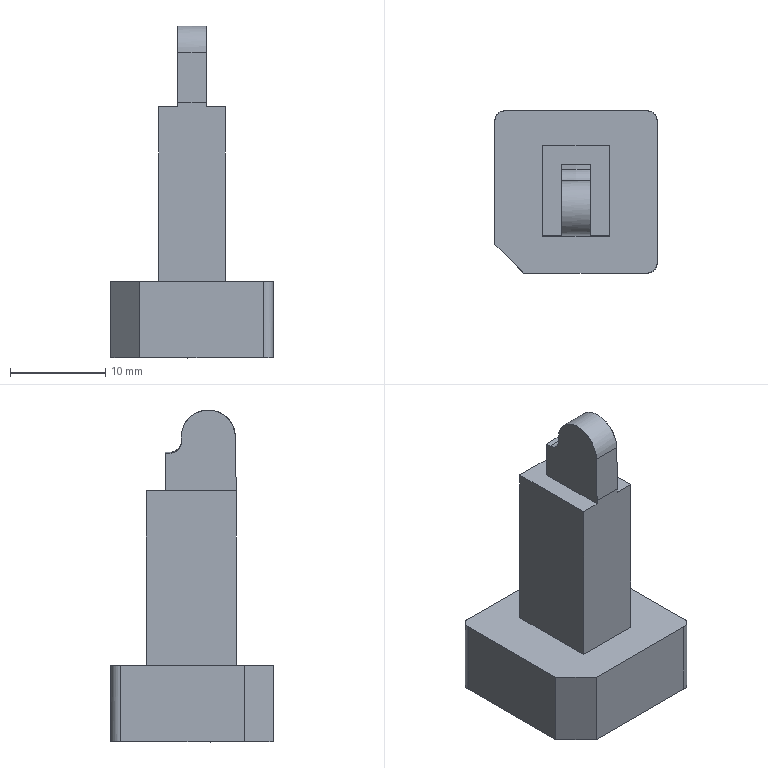NC program | PowerMill | posted with a generic post | part box 17 x 17 x 34.811 mm
Lines 1 to 1077 of 55221:
%
O0001
N104 ( POWERMILL CB  : 2026004.0)
N105 ( POST VER      : 2026.0.0.5161)
N106 ( OPTION FILE   : FANUC)
N107 ( OUTPUT WORKPLANE : WORLD)
N108 (  )
N109 ( TOOL LIST )
N110 (---------------------------------------)
N111 ( NO. | ID        | DIA.| TIP RAD|LENGTH)
N112 (---------------------------------------)
N113 (    1|D10C_1_1_1 |10.0 |  0.0   |90.28 )
N114 (    3|D10_1_1_1  |10.0 |  0.0   |89.96 )
N115 (    4|R1_1_1     | 2.0 |  1.0   |59.84 )
N116 (   14|D4_1_1     | 4.0 |  0.0   |63.76 )
N117 (   13|TEXT_D4_1_1| 4.0 |  0.3   |82.08 )
N118 (---------------------------------------)
N119 (  )
N120 ( NUMBER OF TOOLPATHS: 10.0 )
N121 ( ESTIMATED PROGRAM DURATION: 0 HOURS 6 MIN 45 SEC)
N122 (  )
N123 G00 G21 G80 G40 G17
N124 G90
N125 G54
N126 G53 Z0.0
N127 (---------------)
N128 ( START TOOLPATH : 精公开粗01-扫面平行-D10C )
N129 (---------------)
N130 ( TOOL NO.    :1 )
N131 ( TOOL TYPE   : ENDMILL)
N132 ( TOOL ID     : D10C_1_1_1)
N133 ( TOOL DIA    : 10.0 LENGTH 90.28)
N134 T1
N135 M6
N136 S8000 M03
N137 G00 G90 X0.0 Y0.0
N138 G43 Z10.2 H1
N139
N140 G05 P10000 R4
N141 X11.28 Y11.28
N142 Z1.128
N143 G01 Z-0.072 F6000.0
N144 X-11.28 F10000.0
N145 Y5.64
N146 X11.28
N147 Y0.0
N148 X-11.28
N149 Y-5.64
N150 X11.28
N151 Y-11.28
N152 X-11.28
N153 X-16.28
N154 G00 Z10.2
N155 G05 P0
N156 (---------------)
N157 ( END TOOLPATH : 精公开粗01-扫面平行-D10C )
N158 (---------------)
N159 ( START TOOLPATH : 精公开粗01-外形偏置-D10C )
N160 (---------------)
N161 G00 X0.0 Y0.0915 Z9.878
N162 G05 P10000 R4
N163 X4.7475 Y-17.685
N164 Z0.6945
N165 G01 Z-0.5055 F6000.0
N166 Y-17.1575 F10000.0
N167 G03 X0.0 Y-12.41 I-4.7475 J0.0
N168 G01 X-10.286
N169 G02 X-11.286 Y-11.41 I0.0 J1.0
N170 G01 Y11.593
N171 G02 X-10.286 Y12.593 I1.0 J0.0
N172 G01 X10.286
N173 G02 X11.286 Y11.593 I0.0 J-1.0
N174 G01 Y-11.41
N175 G02 X10.286 Y-12.41 I-1.0 J0.0
N176 G01 X0.0
N177 Y-8.3254
N178 X-1.9336
N179 X-2.707 Y-8.2036
N180 X-3.4804 Y-7.9573
N181 X-4.1209 Y-7.6428
N182 X-5.0273 Y-6.986
N183 X-5.1508 Y-6.8693
N184 X-5.8007 Y-6.1132
N185 X-6.2618 Y-5.3225
N186 X-6.5583 Y-4.5491
N187 X-6.7288 Y-3.7756
N188 X-6.7867 Y-3.0022
N189 Y-0.6819
N190 X-6.7589 Y0.0915
N191 X-6.6303 Y0.8649
N192 X-6.3787 Y1.6384
N193 X-5.9854 Y2.4118
N194 X-5.8007 Y2.6918
N195 X-5.4041 Y3.1852
N196 X-5.0273 Y3.564
N197 X-4.532 Y3.9586
N198 X-4.2538 Y4.1435
N199 X-3.4804 Y4.535
N200 X-2.707 Y4.7817
N201 X-1.9336 Y4.9033
N202 X1.9336
N203 X2.707 Y4.7817
N204 X3.4804 Y4.535
N205 X4.2538 Y4.1435
N206 X4.5319 Y3.9586
N207 X5.0273 Y3.564
N208 X5.404 Y3.1852
N209 X5.8007 Y2.6918
N210 X5.9853 Y2.4118
N211 X6.3781 Y1.6384
N212 X6.6308 Y0.8649
N213 X6.7605 Y0.0915
N214 X6.7867 Y-0.6819
N215 Y-3.0022
N216 X6.7291 Y-3.7756
N217 X6.5741 Y-4.4975
N218 X6.2617 Y-5.3225
N219 X5.8007 Y-6.1132
N220 X5.0273 Y-6.986
N221 X4.1228 Y-7.6428
N222 X3.4804 Y-7.9573
N223 X2.707 Y-8.2036
N224 X1.9336 Y-8.3254
N225 X0.0
N226 Y-12.41
N227 G00 Z3.3111
N228 G01 X4.7475 Y-17.685
N229 G00 Z0.3111
N230 G01 Z-0.8889 F6000.0
N231 Y-17.1575 F10000.0
N232 G03 X0.0 Y-12.41 I-4.7475 J0.0
N233 G01 X-10.286
N234 G02 X-11.286 Y-11.41 I0.0 J1.0
N235 G01 Y11.593
N236 G02 X-10.286 Y12.593 I1.0 J0.0
N237 G01 X10.286
N238 G02 X11.286 Y11.593 I0.0 J-1.0
N239 G01 Y-11.41
N240 G02 X10.286 Y-12.41 I-1.0 J0.0
N241 G01 X1.9336
N242 Y-8.8573
N243 X-1.9336
N244 X-2.707 Y-8.7357
N245 X-3.4804 Y-8.4898
N246 X-4.2538 Y-8.0992
N247 X-5.0273 Y-7.5213
N248 X-5.6368 Y-6.8693
N249 X-5.8007 Y-6.6522
N250 X-6.1452 Y-6.0959
N251 X-6.4857 Y-5.3225
N252 X-6.6923 Y-4.5491
N253 X-6.7815 Y-3.7756
N254 X-6.7825 Y-3.0575
N255 X-6.7867 Y-3.0022
N256 Y-0.6819
N257 X-6.7857 Y-0.6554
N258 X-6.7867 Y0.0915
N259 X-6.7349 Y0.8649
N260 X-6.5741 Y1.6231
N261 X-6.2756 Y2.4118
N262 X-5.8275 Y3.1852
N263 X-5.1707 Y3.9586
N264 X-5.0273 Y4.0949
N265 X-4.2538 Y4.6727
N266 X-3.4804 Y5.0631
N267 X-2.707 Y5.309
N268 X-1.9336 Y5.4306
N269 X1.9336
N270 X2.707 Y5.309
N271 X3.4804 Y5.0631
N272 X4.1542 Y4.7321
N273 X5.0273 Y4.0949
N274 X5.1725 Y3.9586
N275 X5.8007 Y3.2261
N276 X6.2763 Y2.4118
N277 X6.5694 Y1.6384
N278 X6.7353 Y0.8649
N279 X6.7866 Y0.0915
N280 X6.7855 Y-0.6469
N281 X6.7866 Y-0.6819
N282 Y-3.0022
N283 X6.7816 Y-3.0706
N284 X6.7804 Y-3.7756
N285 X6.6926 Y-4.5491
N286 X6.4856 Y-5.3225
N287 X6.1458 Y-6.0959
N288 X5.8007 Y-6.6522
N289 X5.638 Y-6.8693
N290 X5.0273 Y-7.5213
N291 X4.2538 Y-8.0992
N292 X3.6524 Y-8.4162
N293 X2.707 Y-8.7357
N294 X1.9336 Y-8.8573
N295 Y-12.41
N296 X0.0
N297 G00 Z2.9276
N298 G01 X4.7475 Y-17.685
N299 G00 Z-0.0724
N300 G01 Z-1.2724 F6000.0
N301 Y-17.1575 F10000.0
N302 G03 X0.0 Y-12.41 I-4.7475 J0.0
N303 G01 X-10.286
N304 G02 X-11.286 Y-11.41 I0.0 J1.0
N305 G01 Y11.593
N306 G02 X-10.286 Y12.593 I1.0 J0.0
N307 G01 X10.286
N308 G02 X11.286 Y11.593 I0.0 J-1.0
N309 G01 Y-11.41
N310 G02 X10.286 Y-12.41 I-1.0 J0.0
N311 G01 X1.9336
N312 Y-9.2098
N313 X-1.9336
N314 X-2.707 Y-9.0884
N315 X-3.4804 Y-8.843
N316 X-4.2538 Y-8.4532
N317 X-5.0273 Y-7.8767
N318 X-5.2708 Y-7.6428
N319 X-5.8007 Y-7.0103
N320 X-6.3226 Y-6.0959
N321 X-6.5741 Y-5.4128
N322 X-6.7482 Y-4.5491
N323 X-6.7867 Y-3.7756
N324 X-6.7846 Y-3.0294
N325 X-6.7866 Y-3.0022
N326 Y-0.6819
N327 X-6.7857 Y-0.6554
N328 X-6.7867 Y0.0915
N329 X-6.775 Y0.2665
N330 X-6.7732 Y0.8649
N331 X-6.6621 Y1.6384
N332 X-6.5741 Y1.9865
N333 X-6.4298 Y2.4118
N334 X-6.0574 Y3.1852
N335 X-5.8007 Y3.5835
N336 X-5.5058 Y3.9586
N337 X-5.0273 Y4.4498
N338 X-4.6833 Y4.7321
N339 X-4.2538 Y5.0262
N340 X-3.4804 Y5.4158
N341 X-2.707 Y5.6612
N342 X-1.9336 Y5.7826
N343 X1.9336
N344 X2.707 Y5.6612
N345 X3.4804 Y5.4158
N346 X4.2538 Y5.0262
N347 X4.6834 Y4.7321
N348 X5.0273 Y4.4498
N349 X5.5066 Y3.9586
N350 X5.8007 Y3.5835
N351 X6.0582 Y3.1852
N352 X6.4299 Y2.4118
N353 X6.5741 Y1.9865
N354 X6.6618 Y1.6384
N355 X6.7733 Y0.8649
N356 X6.775 Y0.2659
N357 X6.7866 Y0.0915
N358 X6.7854 Y-0.6469
N359 X6.7866 Y-0.6819
N360 Y-3.0022
N361 X6.7846 Y-3.0297
N362 X6.7867 Y-3.7756
N363 X6.7487 Y-4.5491
N364 X6.5995 Y-5.3225
N365 X6.3232 Y-6.0959
N366 X5.8967 Y-6.8693
N367 X5.271 Y-7.6428
N368 X5.0273 Y-7.8767
N369 X4.3133 Y-8.4162
N370 X3.4804 Y-8.843
N371 X2.707 Y-9.0884
N372 X2.1304 Y-9.1896
N373 X1.9336 Y-9.2098
N374 Y-12.41
N375 X0.0
N376 G00 Z2.5442
N377 G01 X4.7475 Y-17.685
N378 G00 Z-0.4558
N379 G01 Z-1.6558 F6000.0
N380 Y-17.1575 F10000.0
N381 G03 X0.0 Y-12.41 I-4.7475 J0.0
N382 G01 X-10.286
N383 G02 X-11.286 Y-11.41 I0.0 J1.0
N384 G01 Y11.593
N385 G02 X-10.286 Y12.593 I1.0 J0.0
N386 G01 X10.286
N387 G02 X11.286 Y11.593 I0.0 J-1.0
N388 G01 Y-11.41
N389 G02 X10.286 Y-12.41 I-1.0 J0.0
N390 G01 X1.9336
N391 Y-9.4549
N392 X-1.9336
N393 X-2.707 Y-9.3335
N394 X-3.4804 Y-9.0882
N395 X-4.2538 Y-8.6991
N396 X-4.6702 Y-8.4162
N397 X-5.0273 Y-8.1236
N398 X-5.4988 Y-7.6428
N399 X-5.8007 Y-7.2587
N400 X-6.0528 Y-6.8693
N401 X-6.428 Y-6.0959
N402 X-6.5741 Y-5.6653
N403 X-6.6617 Y-5.3225
N404 X-6.7729 Y-4.5491
N405 X-6.7741 Y-4.0288
N406 X-6.7867 Y-3.7756
N407 X-6.7845 Y-3.0294
N408 X-6.7866 Y-3.0022
N409 Y-0.6819
N410 X-6.7856 Y-0.6554
N411 X-6.7866 Y0.0915
N412 X-6.7837 Y0.135
N413 X-6.7854 Y0.8649
N414 X-6.7116 Y1.6384
N415 X-6.5741 Y2.2396
N416 X-6.1962 Y3.1852
N417 X-5.708 Y3.9586
N418 X-5.0273 Y4.6974
N419 X-4.2538 Y5.2722
N420 X-3.8294 Y5.5055
N421 X-3.4804 Y5.6612
N422 X-2.707 Y5.9068
N423 X-1.9336 Y6.0281
N424 X1.9336
N425 X2.707 Y5.9068
N426 X3.4804 Y5.6612
N427 X3.829 Y5.5055
N428 X4.2538 Y5.2722
N429 X4.9882 Y4.7321
N430 X5.7074 Y3.9586
N431 X6.1952 Y3.1852
N432 X6.5205 Y2.4118
N433 X6.7123 Y1.6384
N434 X6.7854 Y0.8649
N435 X6.7838 Y0.1332
N436 X6.7865 Y0.0915
N437 X6.7854 Y-0.6469
N438 X6.7865 Y-0.6819
N439 Y-3.0022
N440 X6.7845 Y-3.0297
N441 X6.7867 Y-3.7756
N442 X6.7747 Y-4.0193
N443 X6.7735 Y-4.5491
N444 X6.6618 Y-5.3225
N445 X6.5741 Y-5.6653
N446 X6.428 Y-6.0959
N447 X6.0536 Y-6.8693
N448 X5.8007 Y-7.2587
N449 X5.4991 Y-7.6428
N450 X5.0273 Y-8.1236
N451 X4.6701 Y-8.4162
N452 X4.2538 Y-8.6991
N453 X3.4804 Y-9.0882
N454 X3.2076 Y-9.1896
N455 X2.707 Y-9.3335
N456 X1.9336 Y-9.4549
N457 Y-12.41
N458 X0.0
N459 G00 Z2.1607
N460 G01 X4.7475 Y-17.685
N461 G00 Z-0.8393
N462 G01 Z-2.0393 F6000.0
N463 Y-17.1575 F10000.0
N464 G03 X0.0 Y-12.41 I-4.7475 J0.0
N465 G01 X-10.286
N466 G02 X-11.286 Y-11.41 I0.0 J1.0
N467 G01 Y11.593
N468 G02 X-10.286 Y12.593 I1.0 J0.0
N469 G01 X10.286
N470 G02 X11.286 Y11.593 I0.0 J-1.0
N471 G01 Y-11.41
N472 G02 X10.286 Y-12.41 I-1.0 J0.0
N473 G01 X1.9336
N474 Y-9.6234
N475 X-1.9336
N476 X-2.707 Y-9.5023
N477 X-3.4804 Y-9.2581
N478 X-4.2538 Y-8.87
N479 X-5.0273 Y-8.2941
N480 X-5.6405 Y-7.6428
N481 X-5.8007 Y-7.4317
N482 X-6.1508 Y-6.8693
N483 X-6.4924 Y-6.0959
N484 X-6.6972 Y-5.3225
N485 X-6.7831 Y-4.5491
N486 X-6.7836 Y-3.8369
N487 X-6.7866 Y-3.7756
N488 X-6.7845 Y-3.0294
N489 X-6.7865 Y-3.0022
N490 Y-0.6819
N491 X-6.7857 Y-0.6591
N492 X-6.7859 Y-0.4545
N493 X-6.7866 Y0.0915
N494 X-6.7862 Y0.0969
N495 X-6.7867 Y0.8649
N496 X-6.7393 Y1.6384
N497 X-6.5751 Y2.4118
N498 X-6.2834 Y3.1852
N499 X-5.835 Y3.9586
N500 X-5.1766 Y4.7321
N501 X-5.0273 Y4.8694
N502 X-4.2538 Y5.4448
N503 X-3.4804 Y5.8329
N504 X-2.707 Y6.0776
N505 X-1.9336 Y6.1991
N506 X1.9336
N507 X2.707 Y6.0776
N508 X3.4804 Y5.8329
N509 X4.15 Y5.5055
N510 X5.0273 Y4.8694
N511 X5.1743 Y4.7321
N512 X5.8007 Y4.0069
N513 X6.2828 Y3.1852
N514 X6.5741 Y2.4153
N515 X6.7386 Y1.6384
N516 X6.7867 Y0.8649
N517 X6.7862 Y0.0965
N518 X6.7865 Y0.0915
N519 X6.7859 Y-0.2851
N520 X6.7856 Y-0.6563
N521 X6.7865 Y-0.6819
N522 Y-3.0022
N523 X6.7845 Y-3.0297
N524 X6.7866 Y-3.7756
N525 X6.7833 Y-3.8424
N526 X6.7828 Y-4.5491
N527 X6.6974 Y-5.3225
N528 X6.4921 Y-6.0959
N529 X6.1504 Y-6.8693
N530 X5.8007 Y-7.4317
N531 X5.642 Y-7.6428
N532 X5.0273 Y-8.2941
N533 X4.2538 Y-8.87
N534 X3.6401 Y-9.1896
N535 X2.707 Y-9.5023
N536 X1.9336 Y-9.6234
N537 Y-12.41
N538 X0.0
N539 G00 Z1.7772
N540 G01 X4.7475 Y-17.685
N541 G00 Z-1.2228
N542 G01 Z-2.4228 F6000.0
N543 Y-17.1575 F10000.0
N544 G03 X0.0 Y-12.41 I-4.7475 J0.0
N545 G01 X-0.4032
N546 X-0.3867 Y-9.7437
N547 X-1.9336 Y-9.7341
N548 X-2.707 Y-9.6129
N549 X-3.4804 Y-9.3685
N550 X-3.8822 Y-9.1896
N551 X-4.2538 Y-8.9799
N552 X-5.0166 Y-8.4162
N553 X-5.7274 Y-7.6428
N554 X-6.2105 Y-6.8693
N555 X-6.5304 Y-6.0959
N556 X-6.7161 Y-5.3225
N557 X-6.786 Y-4.5491
N558 X-6.7861 Y-3.7847
N559 X-6.7866 Y-3.7756
N560 X-6.7862 Y-3.6272
N561 Y-3.005
N562 X-6.7865 Y-3.0022
N563 Y-1.1519
N564 X-6.7868 Y0.8649
N565 X-6.7515 Y1.6384
N566 X-6.6077 Y2.4118
N567 X-6.3327 Y3.1852
N568 X-5.9111 Y3.9586
N569 X-5.8007 Y4.1205
N570 X-5.2897 Y4.7321
N571 X-5.0273 Y4.9844
N572 X-4.3381 Y5.5055
N573 X-3.4804 Y5.9464
N574 X-2.707 Y6.1911
N575 X-1.9336 Y6.3121
N576 X-1.1601 Y6.3295
N577 X1.9336 Y6.3121
N578 X2.707 Y6.1911
N579 X3.4804 Y5.9464
N580 X4.2538 Y5.5587
N581 X5.0273 Y4.9844
N582 X5.2902 Y4.7321
N583 X5.9121 Y3.9586
N584 X6.3327 Y3.1852
N585 X6.5741 Y2.5301
N586 X6.7536 Y1.6384
N587 X6.7867 Y0.8649
N588 X6.7864 Y-1.6548
N589 Y-3.0022
N590 X6.7863 Y-3.0043
N591 X6.7862 Y-3.6596
N592 X6.7866 Y-3.7756
N593 X6.7862 Y-3.7827
N594 X6.7861 Y-4.5491
N595 X6.7181 Y-5.3225
N596 X6.5741 Y-5.9579
N597 X6.2089 Y-6.8693
N598 X5.8007 Y-7.5463
N599 X5.0208 Y-8.4162
N600 X4.2538 Y-8.9799
N601 X3.8839 Y-9.1896
N602 X3.4804 Y-9.3685
N603 X2.707 Y-9.6129
N604 X1.9336 Y-9.7341
N605 X1.1601 Y-9.7532
N606 X-0.3867 Y-9.7437
N607 X-0.4032 Y-12.41
N608 X-10.286
N609 G02 X-11.286 Y-11.41 I0.0 J1.0
N610 G01 Y11.593
N611 G02 X-10.286 Y12.593 I1.0 J0.0
N612 G01 X10.286
N613 G02 X11.286 Y11.593 I0.0 J-1.0
N614 G01 Y-11.41
N615 G02 X10.286 Y-12.41 I-1.0 J0.0
N616 G01 X0.0
N617 G00 Z1.3938
N618 G01 X4.7475 Y-17.685
N619 G00 Z-1.6062
N620 G01 Z-2.8062 F6000.0
N621 Y-17.1575 F10000.0
N622 G03 X0.0 Y-12.41 I-4.7475 J0.0
N623 G01 X-10.286
N624 G02 X-11.286 Y-11.41 I0.0 J1.0
N625 G01 Y11.593
N626 G02 X-10.286 Y12.593 I1.0 J0.0
N627 G01 X10.286
N628 G02 X11.286 Y11.593 I0.0 J-1.0
N629 G01 Y-11.41
N630 G02 X10.286 Y-12.41 I-1.0 J0.0
N631 G01 X1.9336
N632 Y-9.7868
N633 X-1.9336
N634 X-2.707 Y-9.6658
N635 X-3.4804 Y-9.4213
N636 X-3.9785 Y-9.1896
N637 X-4.2538 Y-9.0331
N638 X-5.0273 Y-8.459
N639 X-5.7658 Y-7.6428
N640 X-6.2372 Y-6.8693
N641 X-6.547 Y-6.0959
N642 X-6.726 Y-5.3225
N643 X-6.7867 Y-4.5491
N644 X-6.7868 Y0.8649
N645 X-6.7582 Y1.6384
N646 X-6.621 Y2.4118
N647 X-6.3566 Y3.1852
N648 X-5.9462 Y3.9586
N649 X-5.8007 Y4.1729
N650 X-5.3394 Y4.7321
N651 X-5.0273 Y5.0355
N652 X-4.2538 Y5.6095
N653 X-3.4804 Y5.9977
N654 X-2.707 Y6.2422
N655 X-1.9336 Y6.3632
N656 X1.9336
N657 X2.5365 Y6.2789
N658 X3.4804 Y5.9977
N659 X4.2538 Y5.6095
N660 X5.0273 Y5.0355
N661 X5.3394 Y4.7321
N662 X5.8007 Y4.1729
N663 X5.9434 Y3.9586
N664 X6.3572 Y3.1852
N665 X6.5741 Y2.5836
N666 X6.7588 Y1.6384
N667 X6.7867 Y0.8649
N668 Y-4.5491
N669 X6.7258 Y-5.3225
N670 X6.5741 Y-6.0071
N671 X6.2363 Y-6.8693
N672 X5.8007 Y-7.5964
N673 X5.0745 Y-8.4162
N674 X4.2538 Y-9.0331
N675 X3.9784 Y-9.1896
N676 X3.4804 Y-9.4213
N677 X2.707 Y-9.6658
N678 X1.9336 Y-9.7868
N679 Y-12.41
N680 X0.0
N681 G00 Z1.0103
N682 G01 X4.7475 Y-17.685
N683 G00 Z-1.9897
N684 G01 Z-3.1897 F6000.0
N685 Y-17.1575 F10000.0
N686 G03 X0.0 Y-12.41 I-4.7475 J0.0
N687 G01 X-10.286
N688 G02 X-11.286 Y-11.41 I0.0 J1.0
N689 G01 Y11.593
N690 G02 X-10.286 Y12.593 I1.0 J0.0
N691 G01 X10.286
N692 G02 X11.286 Y11.593 I0.0 J-1.0
N693 G01 Y-11.41
N694 G02 X10.286 Y-12.41 I-1.0 J0.0
N695 G01 X1.9972
N696 X1.9336 Y-9.804
N697 X1.1601 Y-9.8229
N698 X-1.9336 Y-9.804
N699 X-2.707 Y-9.6833
N700 X-3.4804 Y-9.4385
N701 X-4.0138 Y-9.1896
N702 X-4.2538 Y-9.0509
N703 X-5.0273 Y-8.4758
N704 X-5.781 Y-7.6428
N705 X-6.2439 Y-6.8693
N706 X-6.5525 Y-6.0959
N707 X-6.7289 Y-5.3225
N708 X-6.7867 Y-4.5491
N709 X-6.7868 Y0.8649
N710 X-6.7617 Y1.6384
N711 X-6.6262 Y2.4118
N712 X-6.3666 Y3.1852
N713 X-5.9559 Y3.9586
N714 X-5.8007 Y4.19
N715 X-5.355 Y4.7321
N716 X-5.0273 Y5.0513
N717 X-4.4419 Y5.5055
N718 X-4.2538 Y5.6222
N719 X-3.4804 Y6.015
N720 X-2.707 Y6.262
N721 X-1.9336 Y6.3806
N722 X-1.1601 Y6.3979
N723 X1.9336 Y6.3806
N724 X2.6145 Y6.2789
N725 X3.4804 Y6.015
N726 X4.2538 Y5.6222
N727 X4.4375 Y5.5055
N728 X5.0273 Y5.0513
N729 X5.3564 Y4.7321
N730 X5.8007 Y4.19
N731 X5.9505 Y3.9586
N732 X6.3617 Y3.1852
N733 X6.4575 Y2.9071
N734 X6.5741 Y2.5836
N735 X6.5809 Y2.5486
N736 X6.628 Y2.4118
N737 X6.7603 Y1.6384
N738 X6.7867 Y0.8649
N739 Y-4.5491
N740 X6.7285 Y-5.3225
N741 X6.5741 Y-6.0252
N742 X6.2427 Y-6.8693
N743 X5.8007 Y-7.6154
N744 X5.0944 Y-8.4162
N745 X4.2538 Y-9.0509
N746 X4.0139 Y-9.1896
N747 X3.4804 Y-9.4385
N748 X2.707 Y-9.6833
N749 X1.9336 Y-9.804
N750 X1.9972 Y-12.41
N751 X0.0
N752 G00 Z0.6269
N753 G01 X4.7475 Y-17.685
N754 G00 Z-2.3731
N755 G01 Z-3.5731 F6000.0
N756 Y-17.1575 F10000.0
N757 G03 X0.0 Y-12.41 I-4.7475 J0.0
N758 G01 X-10.286
N759 G02 X-11.286 Y-11.41 I0.0 J1.0
N760 G01 Y11.593
N761 G02 X-10.286 Y12.593 I1.0 J0.0
N762 G01 X10.286
N763 G02 X11.286 Y11.593 I0.0 J-1.0
N764 G01 Y-11.41
N765 G02 X10.286 Y-12.41 I-1.0 J0.0
N766 G01 X1.9916
N767 X1.9336 Y-9.8123
N768 X1.1601 Y-9.8296
N769 X-1.9336 Y-9.8123
N770 X-2.707 Y-9.6913
N771 X-3.4804 Y-9.4468
N772 X-3.7183 Y-9.3275
N773 X-4.0138 Y-9.1896
N774 X-4.1509 Y-9.1103
N775 X-4.2538 Y-9.0587
N776 X-5.0273 Y-8.4846
N777 X-5.7858 Y-7.6428
N778 X-6.2499 Y-6.8693
N779 X-6.555 Y-6.0959
N780 X-6.7299 Y-5.3225
N781 X-6.7868 Y-4.5491
N782 Y0.8649
N783 X-6.7641 Y1.6384
N784 X-6.631 Y2.4118
N785 X-6.3739 Y3.1852
N786 X-5.9617 Y3.9586
N787 X-5.8007 Y4.1972
N788 X-5.3623 Y4.7321
N789 X-5.0273 Y5.0598
N790 X-4.4543 Y5.5055
N791 X-4.2538 Y5.6339
N792 X-3.4804 Y6.0222
N793 X-2.6533 Y6.2789
N794 X-1.9336 Y6.3877
N795 X-0.3867 Y6.4198
N796 X1.9336 Y6.3877
N797 X2.707 Y6.2713
N798 X3.4804 Y6.0222
N799 X4.2538 Y5.6339
N800 X4.4542 Y5.5055
N801 X5.0273 Y5.0598
N802 X5.3661 Y4.7321
N803 X5.8007 Y4.1972
N804 X5.9617 Y3.9586
N805 X6.368 Y3.1852
N806 X6.6344 Y2.4118
N807 X6.7618 Y1.6384
N808 X6.7867 Y0.8649
N809 Y-4.5491
N810 X6.7299 Y-5.3225
N811 X6.5741 Y-6.0328
N812 X6.2491 Y-6.8693
N813 X5.7858 Y-7.6428
N814 X5.1022 Y-8.4162
N815 X4.2538 Y-9.0587
N816 X4.026 Y-9.1896
N817 X3.4804 Y-9.4468
N818 X2.707 Y-9.6913
N819 X1.9336 Y-9.8123
N820 X1.9916 Y-12.41
N821 X0.0
N822 G00 Z0.2434
N823 G01 X4.7475 Y-17.685
N824 G00 Z-2.7566
N825 G01 Z-3.9566 F6000.0
N826 Y-17.1575 F10000.0
N827 G03 X0.0 Y-12.41 I-4.7475 J0.0
N828 G01 X-10.286
N829 G02 X-11.286 Y-11.41 I0.0 J1.0
N830 G01 Y11.593
N831 G02 X-10.286 Y12.593 I1.0 J0.0
N832 G01 X10.286
N833 G02 X11.286 Y11.593 I0.0 J-1.0
N834 G01 Y-11.41
N835 G02 X10.286 Y-12.41 I-1.0 J0.0
N836 G01 X1.9915
N837 X1.9336 Y-9.819
N838 X1.1601 Y-9.8363
N839 X-1.9336 Y-9.819
N840 X-2.707 Y-9.698
N841 X-3.4804 Y-9.4535
N842 X-3.9095 Y-9.2382
N843 X-4.0137 Y-9.1895
N844 X-4.0621 Y-9.1616
N845 X-4.2538 Y-9.0653
N846 X-5.0273 Y-8.4913
N847 X-5.7907 Y-7.6428
N848 X-6.2531 Y-6.8693
N849 X-6.5573 Y-6.0959
N850 X-6.7309 Y-5.3225
N851 X-6.7868 Y-4.5491
N852 Y0.8649
N853 X-6.7695 Y1.6384
N854 X-6.6488 Y2.4118
N855 X-6.4052 Y3.1852
N856 X-6.0176 Y3.9586
N857 X-5.8007 Y4.288
N858 X-5.4452 Y4.7321
N859 X-5.0273 Y5.1516
N860 X-4.5854 Y5.5055
N861 X-4.2538 Y5.7263
N862 X-3.4804 Y6.1149
N863 X-2.707 Y6.3597
N864 X-1.9336 Y6.4808
N865 X-1.1601 Y6.5158
N866 X0.3867 Y6.5438
N867 X1.9336 Y6.4808
N868 X2.707 Y6.3597
N869 X3.4804 Y6.1149
N870 X4.2538 Y5.7263
N871 X4.5859 Y5.5055
N872 X5.0273 Y5.1516
N873 X5.4456 Y4.7321
N874 X5.8007 Y4.288
N875 X6.0178 Y3.9586
N876 X6.4047 Y3.1852
N877 X6.6487 Y2.4118
N878 X6.7705 Y1.6384
N879 X6.7712 Y1.3453
N880 X6.7867 Y0.8649
N881 Y-4.527
N882 Y-4.5491
N883 X6.7309 Y-5.3225
N884 X6.5741 Y-6.0395
N885 X6.2531 Y-6.8693
N886 X5.8007 Y-7.6288
N887 X5.1094 Y-8.4162
N888 X4.2538 Y-9.0653
N889 X4.0379 Y-9.1896
N890 X3.4804 Y-9.4535
N891 X2.707 Y-9.698
N892 X1.9336 Y-9.819
N893 X1.9915 Y-12.41
N894 X0.0
N895 G00 Z-0.1401
N896 G01 X4.7475 Y-17.685
N897 G00 Z-3.1401
N898 G01 Z-4.3401 F6000.0
N899 Y-17.1575 F10000.0
N900 G03 X0.0 Y-12.41 I-4.7475 J0.0
N901 G01 X-10.286
N902 G02 X-11.286 Y-11.41 I0.0 J1.0
N903 G01 Y11.593
N904 G02 X-10.286 Y12.593 I1.0 J0.0
N905 G01 X10.286
N906 G02 X11.286 Y11.593 I0.0 J-1.0
N907 G01 Y-11.41
N908 G02 X10.286 Y-12.41 I-1.0 J0.0
N909 G01 X1.9913
N910 X1.9336 Y-9.8257
N911 X1.1601 Y-9.843
N912 X-1.9336 Y-9.8257
N913 X-2.707 Y-9.7047
N914 X-3.4804 Y-9.4602
N915 X-4.2538 Y-9.072
N916 X-5.0273 Y-8.498
N917 X-5.7955 Y-7.6428
N918 X-6.2564 Y-6.8693
N919 X-6.5593 Y-6.0959
N920 X-6.7318 Y-5.3225
N921 X-6.7868 Y-4.5491
N922 X-6.7867 Y-4.4591
N923 Y0.8649
N924 X-6.7833 Y1.0184
N925 X-6.7829 Y1.6384
N926 X-6.6992 Y2.4118
N927 X-6.4954 Y3.1852
N928 X-6.1588 Y3.9586
N929 X-5.8007 Y4.5424
N930 X-5.6586 Y4.7321
N931 X-5.0273 Y5.4104
N932 X-4.2538 Y5.9901
N933 X-3.4804 Y6.3788
N934 X-2.707 Y6.6244
N935 X-1.9336 Y6.7493
N936 X-1.1601 Y6.8271
N937 X-0.3867 Y6.8678
N938 X0.3867
N939 X1.1601 Y6.8271
N940 X1.9336 Y6.7493
N941 X2.707 Y6.6244
N942 X3.4804 Y6.3788
N943 X4.2538 Y5.9901
N944 X4.9169 Y5.5055
N945 X5.6598 Y4.7321
N946 X5.8007 Y4.5424
N947 X6.1608 Y3.9586
N948 X6.4951 Y3.1852
N949 X6.7002 Y2.4118
N950 X6.7827 Y1.6384
N951 X6.7831 Y0.9746
N952 X6.7866 Y0.8649
N953 Y-4.3739
N954 X6.7867 Y-4.5491
N955 X6.7318 Y-5.3225
N956 X6.5741 Y-6.0462
N957 X6.2564 Y-6.8693
N958 X5.8007 Y-7.6355
N959 X5.1166 Y-8.4162
N960 X4.2538 Y-9.072
N961 X4.0498 Y-9.1896
N962 X3.4804 Y-9.4602
N963 X2.707 Y-9.7047
N964 X1.9336 Y-9.8257
N965 X1.9913 Y-12.41
N966 X0.0
N967 G00 Z-0.5235
N968 G01 X4.7475 Y-17.685
N969 G00 Z-3.5235
N970 G01 Z-4.7235 F6000.0
N971 Y-17.1575 F10000.0
N972 G03 X0.0 Y-12.41 I-4.7475 J0.0
N973 G01 X-10.286
N974 G02 X-11.286 Y-11.41 I0.0 J1.0
N975 G01 Y11.593
N976 G02 X-10.286 Y12.593 I1.0 J0.0
N977 G01 X10.286
N978 G02 X11.286 Y11.593 I0.0 J-1.0
N979 G01 Y-11.41
N980 G02 X10.286 Y-12.41 I-1.0 J0.0
N981 G01 X1.9912
N982 X1.9336 Y-9.8324
N983 X1.1601 Y-9.8496
N984 X-1.9336 Y-9.8324
N985 X-2.707 Y-9.7114
N986 X-3.4804 Y-9.4669
N987 X-4.2538 Y-9.0787
N988 X-5.0273 Y-8.5047
N989 X-5.8003 Y-7.6428
N990 X-6.2596 Y-6.8693
N991 X-6.5613 Y-6.0959
N992 X-6.7328 Y-5.3225
N993 X-6.7868 Y-4.5491
N994 X-6.7867 Y2.4118
N995 X-6.7738 Y3.1852
N996 X-6.6616 Y3.9586
N997 X-6.5741 Y4.2995
N998 X-6.4268 Y4.7321
N999 X-6.0505 Y5.5055
N1000 X-5.8007 Y5.8887
N1001 X-5.4927 Y6.2789
N1002 X-5.0273 Y6.7513
N1003 X-4.6586 Y7.0523
N1004 X-4.2538 Y7.3253
N1005 X-3.4804 Y7.7135
N1006 X-3.175 Y7.8258
N1007 X-2.707 Y7.958
N1008 X-1.9336 Y8.0789
N1009 X-1.1601 Y8.0962
N1010 X1.9336 Y8.0789
N1011 X2.707 Y7.958
N1012 X3.175 Y7.8258
N1013 X3.4804 Y7.7135
N1014 X4.2538 Y7.3253
N1015 X4.6585 Y7.0523
N1016 X5.0273 Y6.7513
N1017 X5.4928 Y6.2789
N1018 X5.8007 Y5.8887
N1019 X6.0505 Y5.5055
N1020 X6.4269 Y4.7321
N1021 X6.5741 Y4.2995
N1022 X6.6617 Y3.9586
N1023 X6.7738 Y3.1852
N1024 X6.7867 Y2.4118
N1025 Y-4.5491
N1026 X6.7328 Y-5.3225
N1027 X6.5741 Y-6.0529
N1028 X6.2596 Y-6.8693
N1029 X5.8007 Y-7.6422
N1030 X5.1237 Y-8.4162
N1031 X4.2538 Y-9.0787
N1032 X4.0617 Y-9.1896
N1033 X3.4804 Y-9.4669
N1034 X2.707 Y-9.7114
N1035 X1.9336 Y-9.8324
N1036 X1.9912 Y-12.41
N1037 X0.0
N1038 G00 Z-0.907
N1039 G01 X4.7475 Y-17.685
N1040 G00 Z-3.907
N1041 G01 Z-5.107 F6000.0
N1042 Y-17.1575 F10000.0
N1043 G03 X0.0 Y-12.41 I-4.7475 J0.0
N1044 G01 X-10.286
N1045 G02 X-11.286 Y-11.41 I0.0 J1.0
N1046 G01 Y11.593
N1047 G02 X-10.286 Y12.593 I1.0 J0.0
N1048 G01 X10.286
N1049 G02 X11.286 Y11.593 I0.0 J-1.0
N1050 G01 Y-11.41
N1051 G02 X10.286 Y-12.41 I-1.0 J0.0
N1052 G01 X1.991
N1053 X1.9336 Y-9.8391
N1054 X1.1601 Y-9.8563
N1055 X-1.9336 Y-9.8391
N1056 X-2.707 Y-9.7181
N1057 X-3.4804 Y-9.4736
N1058 X-4.2538 Y-9.0854
N1059 X-5.0273 Y-8.5113
N1060 X-5.8007 Y-7.6489
N1061 X-6.2628 Y-6.8693
N1062 X-6.5634 Y-6.0959
N1063 X-6.7338 Y-5.3225
N1064 X-6.7868 Y-4.5491
N1065 Y2.4118
N1066 X-6.7738 Y3.1852
N1067 X-6.6616 Y3.9586
N1068 X-6.5741 Y4.2995
N1069 X-6.4269 Y4.7321
N1070 X-6.0506 Y5.5055
N1071 X-5.8007 Y5.8887
N1072 X-5.4927 Y6.2789
N1073 X-5.0273 Y6.7513
N1074 X-4.6586 Y7.0523
N1075 X-4.2538 Y7.3253
N1076 X-3.4804 Y7.7135
N1077 X-3.4792 Y7.7139
N1078 X-3.175 Y7.8257
N1079 X-2.7089 Y7.9574
N1080 X-2.707 Y7.958
N1081 X-1.9336 Y8.0789
N1082 X-1.1601 Y8.0962
N1083 X1.9336 Y8.0789
N1084 X2.707 Y7.958
N1085 X2.7089 Y7.9574
N1086 X3.175 Y7.8257
N1087 X3.4792 Y7.7139
N1088 X3.4804 Y7.7135
N1089 X4.2538 Y7.3253
N1090 X4.6585 Y7.0523
N1091 X5.0273 Y6.7513
N1092 X5.4928 Y6.2789
N1093 X5.8007 Y5.8887
N1094 X6.0505 Y5.5055
N1095 X6.4269 Y4.7321
N1096 X6.5741 Y4.2995
N1097 X6.6617 Y3.9586
N1098 X6.7738 Y3.1852
N1099 X6.7867 Y2.4118
N1100 Y-4.5491
N1101 X6.7338 Y-5.3225
N1102 X6.5741 Y-6.0596
N1103 X6.2628 Y-6.8693
N1104 X5.805 Y-7.6428
N1105 X5.1308 Y-8.4162
N1106 X4.2538 Y-9.0854
N1107 X4.0736 Y-9.1896
N1108 X3.4804 Y-9.4736
N1109 X2.707 Y-9.7181
N1110 X1.9336 Y-9.8391
N1111 X1.991 Y-12.41
N1112 X0.0
N1113 G00 Z-1.2904
N1114 G01 X4.7475 Y-17.685
N1115 G00 Z-4.2905
N1116 G01 Z-5.4904 F6000.0
N1117 Y-17.1575 F10000.0
N1118 G03 X0.0 Y-12.41 I-4.7475 J0.0
N1119 G01 X-10.286
N1120 G02 X-11.286 Y-11.41 I0.0 J1.0
N1121 G01 Y11.593
N1122 G02 X-10.286 Y12.593 I1.0 J0.0
N1123 G01 X10.286
N1124 G02 X11.286 Y11.593 I0.0 J-1.0
N1125 G01 Y-11.41
N1126 G02 X10.286 Y-12.41 I-1.0 J0.0
N1127 G01 X1.9909
N1128 X1.9336 Y-9.8458
N1129 X1.1601 Y-9.863
N1130 X-1.9336 Y-9.8458
N1131 X-2.707 Y-9.7248
N1132 X-3.4804 Y-9.4803
N1133 X-4.2538 Y-9.0921
N1134 X-5.0273 Y-8.518
N1135 X-5.8007 Y-7.6556
N1136 X-6.2661 Y-6.8693
N1137 X-6.5654 Y-6.0959
N1138 X-6.7347 Y-5.3225
N1139 X-6.7868 Y-4.5491
N1140 Y2.4118
N1141 X-6.7738 Y3.1852
N1142 X-6.6617 Y3.9586
N1143 X-6.5741 Y4.2995
N1144 X-6.4269 Y4.7321
N1145 X-6.0506 Y5.5055
N1146 X-5.8007 Y5.8887
N1147 X-5.4927 Y6.2789
N1148 X-5.0273 Y6.7513
N1149 X-4.6586 Y7.0523
N1150 X-4.2538 Y7.3253
N1151 X-3.4804 Y7.7135
N1152 X-3.478 Y7.7143
N1153 X-3.175 Y7.8257
N1154 X-2.7108 Y7.9568
N1155 X-2.707 Y7.958
N1156 X-1.9336 Y8.079
N1157 X-1.1601 Y8.0962
N1158 X1.9336 Y8.079
N1159 X2.707 Y7.958
N1160 X2.7108 Y7.9568
N1161 X3.175 Y7.8257
N1162 X3.478 Y7.7143
N1163 X3.4804 Y7.7135
N1164 X4.2538 Y7.3253
N1165 X4.6585 Y7.0523
N1166 X5.0273 Y6.7513
N1167 X5.4928 Y6.2789
N1168 X5.8007 Y5.8887
N1169 X6.0505 Y5.5055
N1170 X6.4269 Y4.7321
N1171 X6.5741 Y4.2995
N1172 X6.6617 Y3.9586
N1173 X6.7738 Y3.1852
N1174 X6.7867 Y2.4118